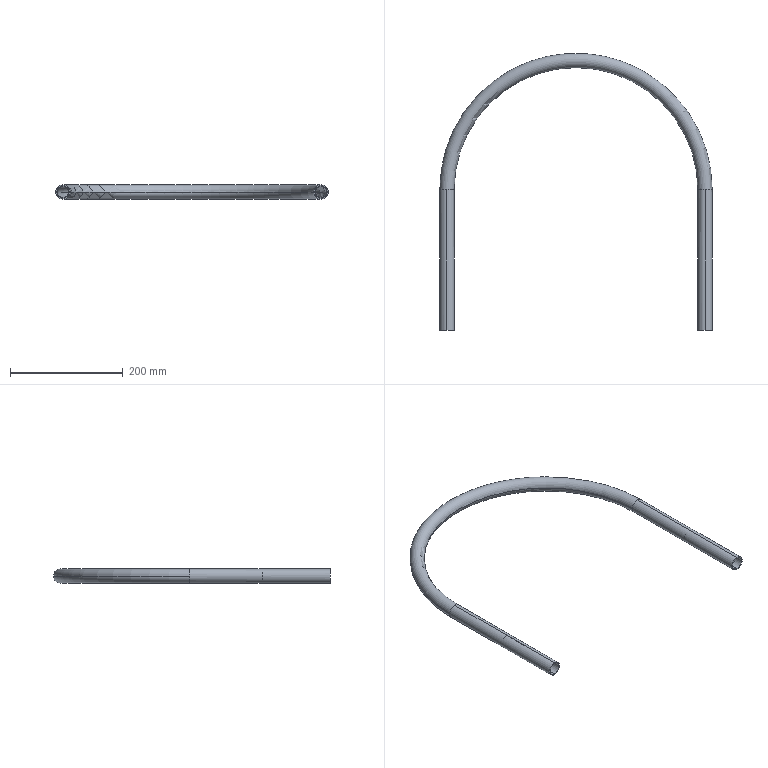Part | STEP file | 51E-01212JG10 | 1 solid | 20 faces | box 483.4 x 491.7 x 25.4 mm | volume 222157 mm3 | cylinder 12 | torus 4 | plane 4 | commonest cylinder face diameters 19.8 x4 25.4 x4 22.2 x2 22.5 x2
STEP:
#1=CARTESIAN_POINT('',(-238.9,250.,0.));
#2=VERTEX_POINT('',#1);
#3=CARTESIAN_POINT('',(-229.,250.,9.9));
#4=VERTEX_POINT('',#3);
#5=CARTESIAN_POINT('',(-229.,250.,0.));
#6=DIRECTION('',(0.,-1.,0.));
#7=AXIS2_PLACEMENT_3D('',#5,#6,$);
#8=CIRCLE('',#7,9.9);
#9=EDGE_CURVE('',#2,#4,#8,.F.);
#10=ORIENTED_EDGE('',*,*,#9,.F.);
#11=CARTESIAN_POINT('',(238.9,250.,0.));
#12=VERTEX_POINT('',#11);
#13=CARTESIAN_POINT('',(0.,250.,0.));
#14=DIRECTION('',(0.,0.,-1.));
#15=AXIS2_PLACEMENT_3D('',#13,#14,$);
#16=CIRCLE('',#15,238.9);
#17=EDGE_CURVE('',#2,#12,#16,.T.);
#18=ORIENTED_EDGE('',*,*,#17,.T.);
#19=CARTESIAN_POINT('',(229.,250.,9.9));
#20=VERTEX_POINT('',#19);
#21=CARTESIAN_POINT('',(229.,250.,0.));
#22=DIRECTION('',(0.,1.,0.));
#23=AXIS2_PLACEMENT_3D('',#21,#22,$);
#24=CIRCLE('',#23,9.9);
#25=EDGE_CURVE('',#12,#20,#24,.F.);
#26=ORIENTED_EDGE('',*,*,#25,.T.);
#27=CARTESIAN_POINT('',(219.1,250.,0.));
#28=VERTEX_POINT('',#27);
#29=CARTESIAN_POINT('',(229.,250.,0.));
#30=DIRECTION('',(0.,1.,0.));
#31=AXIS2_PLACEMENT_3D('',#29,#30,$);
#32=CIRCLE('',#31,9.9);
#33=EDGE_CURVE('',#20,#28,#32,.F.);
#34=ORIENTED_EDGE('',*,*,#33,.T.);
#35=CARTESIAN_POINT('',(-219.1,250.,0.));
#36=VERTEX_POINT('',#35);
#37=CARTESIAN_POINT('',(0.,250.,0.));
#38=DIRECTION('',(0.,0.,-1.));
#39=AXIS2_PLACEMENT_3D('',#37,#38,$);
#40=CIRCLE('',#39,219.1);
#41=EDGE_CURVE('',#36,#28,#40,.T.);
#42=ORIENTED_EDGE('',*,*,#41,.F.);
#43=CARTESIAN_POINT('',(-229.,250.,0.));
#44=DIRECTION('',(0.,-1.,0.));
#45=AXIS2_PLACEMENT_3D('',#43,#44,$);
#46=CIRCLE('',#45,9.9);
#47=EDGE_CURVE('',#4,#36,#46,.F.);
#48=ORIENTED_EDGE('',*,*,#47,.F.);
#49=EDGE_LOOP('',(#10,#18,#26,#34,#42,#48));
#50=FACE_OUTER_BOUND('',#49,.T.);
#51=CARTESIAN_POINT('',(0.,250.,0.));
#52=DIRECTION('',(0.,0.,-1.));
#53=DIRECTION('',(-1.,0.,0.));
#54=AXIS2_PLACEMENT_3D('',#51,#52,#53);
#55=TOROIDAL_SURFACE('',#54,229.,9.9);
#56=ADVANCED_FACE('',(#50),#55,.F.);
#57=CARTESIAN_POINT('',(-229.,250.,-9.9));
#58=VERTEX_POINT('',#57);
#59=CARTESIAN_POINT('',(-229.,250.,0.));
#60=DIRECTION('',(0.,-1.,0.));
#61=AXIS2_PLACEMENT_3D('',#59,#60,$);
#62=CIRCLE('',#61,9.9);
#63=EDGE_CURVE('',#58,#2,#62,.F.);
#64=ORIENTED_EDGE('',*,*,#63,.T.);
#65=ORIENTED_EDGE('',*,*,#9,.T.);
#66=CARTESIAN_POINT('',(-229.,120.,9.9));
#67=VERTEX_POINT('',#66);
#68=CARTESIAN_POINT('',(-229.,250.,9.9));
#69=DIRECTION('',(0.,-1.,0.));
#70=VECTOR('',#69,1.);
#71=LINE('',#68,#70);
#72=EDGE_CURVE('',#4,#67,#71,.T.);
#73=ORIENTED_EDGE('',*,*,#72,.T.);
#74=CARTESIAN_POINT('',(-229.,120.,-9.9));
#75=VERTEX_POINT('',#74);
#76=CARTESIAN_POINT('',(-229.,120.,0.));
#77=DIRECTION('',(0.,-1.,0.));
#78=AXIS2_PLACEMENT_3D('',#76,#77,$);
#79=CIRCLE('',#78,9.9);
#80=EDGE_CURVE('',#75,#67,#79,.F.);
#81=ORIENTED_EDGE('',*,*,#80,.F.);
#82=CARTESIAN_POINT('',(-229.,250.,-9.9));
#83=DIRECTION('',(0.,-1.,0.));
#84=VECTOR('',#83,1.);
#85=LINE('',#82,#84);
#86=EDGE_CURVE('',#58,#75,#85,.T.);
#87=ORIENTED_EDGE('',*,*,#86,.F.);
#88=EDGE_LOOP('',(#64,#65,#73,#81,#87));
#89=FACE_OUTER_BOUND('',#88,.T.);
#90=CARTESIAN_POINT('',(-229.,250.,0.));
#91=DIRECTION('',(0.,-1.,0.));
#92=DIRECTION('',(0.,0.,1.));
#93=AXIS2_PLACEMENT_3D('',#90,#91,#92);
#94=CYLINDRICAL_SURFACE('',#93,9.9);
#95=ADVANCED_FACE('',(#89),#94,.F.);
#96=ORIENTED_EDGE('',*,*,#17,.F.);
#97=ORIENTED_EDGE('',*,*,#63,.F.);
#98=CARTESIAN_POINT('',(-229.,250.,0.));
#99=DIRECTION('',(0.,-1.,0.));
#100=AXIS2_PLACEMENT_3D('',#98,#99,$);
#101=CIRCLE('',#100,9.9);
#102=EDGE_CURVE('',#36,#58,#101,.F.);
#103=ORIENTED_EDGE('',*,*,#102,.F.);
#104=ORIENTED_EDGE('',*,*,#41,.T.);
#105=CARTESIAN_POINT('',(229.,250.,-9.9));
#106=VERTEX_POINT('',#105);
#107=CARTESIAN_POINT('',(229.,250.,0.));
#108=DIRECTION('',(0.,1.,0.));
#109=AXIS2_PLACEMENT_3D('',#107,#108,$);
#110=CIRCLE('',#109,9.9);
#111=EDGE_CURVE('',#28,#106,#110,.F.);
#112=ORIENTED_EDGE('',*,*,#111,.T.);
#113=CARTESIAN_POINT('',(229.,250.,0.));
#114=DIRECTION('',(0.,1.,0.));
#115=AXIS2_PLACEMENT_3D('',#113,#114,$);
#116=CIRCLE('',#115,9.9);
#117=EDGE_CURVE('',#106,#12,#116,.F.);
#118=ORIENTED_EDGE('',*,*,#117,.T.);
#119=EDGE_LOOP('',(#96,#97,#103,#104,#112,#118));
#120=FACE_OUTER_BOUND('',#119,.T.);
#121=CARTESIAN_POINT('',(0.,250.,0.));
#122=DIRECTION('',(0.,0.,-1.));
#123=DIRECTION('',(-1.,0.,0.));
#124=AXIS2_PLACEMENT_3D('',#121,#122,#123);
#125=TOROIDAL_SURFACE('',#124,229.,9.9);
#126=ADVANCED_FACE('',(#120),#125,.F.);
#127=CARTESIAN_POINT('',(229.,120.,9.9));
#128=VERTEX_POINT('',#127);
#129=CARTESIAN_POINT('',(229.,250.,9.9));
#130=DIRECTION('',(0.,-1.,0.));
#131=VECTOR('',#130,1.);
#132=LINE('',#129,#131);
#133=EDGE_CURVE('',#20,#128,#132,.T.);
#134=ORIENTED_EDGE('',*,*,#133,.F.);
#135=ORIENTED_EDGE('',*,*,#25,.F.);
#136=ORIENTED_EDGE('',*,*,#117,.F.);
#137=CARTESIAN_POINT('',(229.,120.,-9.9));
#138=VERTEX_POINT('',#137);
#139=CARTESIAN_POINT('',(229.,250.,-9.9));
#140=DIRECTION('',(0.,-1.,0.));
#141=VECTOR('',#140,1.);
#142=LINE('',#139,#141);
#143=EDGE_CURVE('',#106,#138,#142,.T.);
#144=ORIENTED_EDGE('',*,*,#143,.T.);
#145=CARTESIAN_POINT('',(229.,120.,0.));
#146=DIRECTION('',(0.,-1.,0.));
#147=AXIS2_PLACEMENT_3D('',#145,#146,$);
#148=CIRCLE('',#147,9.9);
#149=EDGE_CURVE('',#138,#128,#148,.T.);
#150=ORIENTED_EDGE('',*,*,#149,.T.);
#151=EDGE_LOOP('',(#134,#135,#136,#144,#150));
#152=FACE_OUTER_BOUND('',#151,.T.);
#153=CARTESIAN_POINT('',(229.,250.,0.));
#154=DIRECTION('',(0.,-1.,0.));
#155=DIRECTION('',(0.,0.,-1.));
#156=AXIS2_PLACEMENT_3D('',#153,#154,#155);
#157=CYLINDRICAL_SURFACE('',#156,9.9);
#158=ADVANCED_FACE('',(#152),#157,.F.);
#159=ORIENTED_EDGE('',*,*,#33,.F.);
#160=ORIENTED_EDGE('',*,*,#133,.T.);
#161=CARTESIAN_POINT('',(229.,120.,0.));
#162=DIRECTION('',(0.,-1.,0.));
#163=AXIS2_PLACEMENT_3D('',#161,#162,$);
#164=CIRCLE('',#163,9.9);
#165=EDGE_CURVE('',#128,#138,#164,.T.);
#166=ORIENTED_EDGE('',*,*,#165,.T.);
#167=ORIENTED_EDGE('',*,*,#143,.F.);
#168=ORIENTED_EDGE('',*,*,#111,.F.);
#169=EDGE_LOOP('',(#159,#160,#166,#167,#168));
#170=FACE_OUTER_BOUND('',#169,.T.);
#171=CARTESIAN_POINT('',(229.,250.,0.));
#172=DIRECTION('',(0.,-1.,0.));
#173=DIRECTION('',(0.,0.,1.));
#174=AXIS2_PLACEMENT_3D('',#171,#172,#173);
#175=CYLINDRICAL_SURFACE('',#174,9.9);
#176=ADVANCED_FACE('',(#170),#175,.F.);
#177=ORIENTED_EDGE('',*,*,#72,.F.);
#178=ORIENTED_EDGE('',*,*,#47,.T.);
#179=ORIENTED_EDGE('',*,*,#102,.T.);
#180=ORIENTED_EDGE('',*,*,#86,.T.);
#181=CARTESIAN_POINT('',(-229.,120.,0.));
#182=DIRECTION('',(0.,-1.,0.));
#183=AXIS2_PLACEMENT_3D('',#181,#182,$);
#184=CIRCLE('',#183,9.9);
#185=EDGE_CURVE('',#67,#75,#184,.F.);
#186=ORIENTED_EDGE('',*,*,#185,.F.);
#187=EDGE_LOOP('',(#177,#178,#179,#180,#186));
#188=FACE_OUTER_BOUND('',#187,.T.);
#189=CARTESIAN_POINT('',(-229.,250.,0.));
#190=DIRECTION('',(0.,-1.,0.));
#191=DIRECTION('',(0.,0.,-1.));
#192=AXIS2_PLACEMENT_3D('',#189,#190,#191);
#193=CYLINDRICAL_SURFACE('',#192,9.9);
#194=ADVANCED_FACE('',(#188),#193,.F.);
#195=CARTESIAN_POINT('',(-229.,120.,-11.1));
#196=VERTEX_POINT('',#195);
#197=CARTESIAN_POINT('',(-229.,120.,11.1));
#198=VERTEX_POINT('',#197);
#199=CARTESIAN_POINT('',(-229.,120.,0.));
#200=DIRECTION('',(0.,1.,0.));
#201=AXIS2_PLACEMENT_3D('',#199,#200,$);
#202=CIRCLE('',#201,11.1);
#203=EDGE_CURVE('',#196,#198,#202,.T.);
#204=ORIENTED_EDGE('',*,*,#203,.F.);
#205=CARTESIAN_POINT('',(-229.,120.,0.));
#206=DIRECTION('',(0.,1.,0.));
#207=AXIS2_PLACEMENT_3D('',#205,#206,$);
#208=CIRCLE('',#207,11.1);
#209=EDGE_CURVE('',#198,#196,#208,.T.);
#210=ORIENTED_EDGE('',*,*,#209,.F.);
#211=EDGE_LOOP('',(#204,#210));
#212=FACE_OUTER_BOUND('',#211,.T.);
#213=ORIENTED_EDGE('',*,*,#80,.T.);
#214=ORIENTED_EDGE('',*,*,#185,.T.);
#215=EDGE_LOOP('',(#213,#214));
#216=FACE_BOUND('',#215,.T.);
#217=CARTESIAN_POINT('',(-229.,120.,0.));
#218=DIRECTION('',(0.,1.,0.));
#219=DIRECTION('',(0.,0.,1.));
#220=AXIS2_PLACEMENT_3D('',#217,#218,#219);
#221=PLANE('',#220);
#222=ADVANCED_FACE('',(#212,#216),#221,.F.);
#223=CARTESIAN_POINT('',(229.,120.,-11.25));
#224=VERTEX_POINT('',#223);
#225=CARTESIAN_POINT('',(229.,120.,11.25));
#226=VERTEX_POINT('',#225);
#227=CARTESIAN_POINT('',(229.,120.,0.));
#228=DIRECTION('',(0.,1.,0.));
#229=AXIS2_PLACEMENT_3D('',#227,#228,$);
#230=CIRCLE('',#229,11.25);
#231=EDGE_CURVE('',#224,#226,#230,.T.);
#232=ORIENTED_EDGE('',*,*,#231,.F.);
#233=CARTESIAN_POINT('',(229.,120.,0.));
#234=DIRECTION('',(0.,1.,0.));
#235=AXIS2_PLACEMENT_3D('',#233,#234,$);
#236=CIRCLE('',#235,11.25);
#237=EDGE_CURVE('',#226,#224,#236,.T.);
#238=ORIENTED_EDGE('',*,*,#237,.F.);
#239=EDGE_LOOP('',(#232,#238));
#240=FACE_OUTER_BOUND('',#239,.T.);
#241=ORIENTED_EDGE('',*,*,#149,.F.);
#242=ORIENTED_EDGE('',*,*,#165,.F.);
#243=EDGE_LOOP('',(#241,#242));
#244=FACE_BOUND('',#243,.T.);
#245=CARTESIAN_POINT('',(229.,120.,0.));
#246=DIRECTION('',(0.,1.,0.));
#247=DIRECTION('',(0.,0.,1.));
#248=AXIS2_PLACEMENT_3D('',#245,#246,#247);
#249=PLANE('',#248);
#250=ADVANCED_FACE('',(#240,#244),#249,.F.);
#251=ORIENTED_EDGE('',*,*,#203,.T.);
#252=CARTESIAN_POINT('',(-229.,0.,11.1));
#253=VERTEX_POINT('',#252);
#254=CARTESIAN_POINT('',(-229.,120.,11.1));
#255=DIRECTION('',(0.,-1.,0.));
#256=VECTOR('',#255,1.);
#257=LINE('',#254,#256);
#258=EDGE_CURVE('',#198,#253,#257,.T.);
#259=ORIENTED_EDGE('',*,*,#258,.T.);
#260=CARTESIAN_POINT('',(-229.,0.,-11.1));
#261=VERTEX_POINT('',#260);
#262=CARTESIAN_POINT('',(-229.,0.,0.));
#263=DIRECTION('',(0.,-1.,0.));
#264=AXIS2_PLACEMENT_3D('',#262,#263,$);
#265=CIRCLE('',#264,11.1);
#266=EDGE_CURVE('',#261,#253,#265,.F.);
#267=ORIENTED_EDGE('',*,*,#266,.F.);
#268=CARTESIAN_POINT('',(-229.,120.,-11.1));
#269=DIRECTION('',(0.,-1.,0.));
#270=VECTOR('',#269,1.);
#271=LINE('',#268,#270);
#272=EDGE_CURVE('',#196,#261,#271,.T.);
#273=ORIENTED_EDGE('',*,*,#272,.F.);
#274=EDGE_LOOP('',(#251,#259,#267,#273));
#275=FACE_OUTER_BOUND('',#274,.T.);
#276=CARTESIAN_POINT('',(-229.,120.,0.));
#277=DIRECTION('',(0.,-1.,0.));
#278=DIRECTION('',(0.,0.,1.));
#279=AXIS2_PLACEMENT_3D('',#276,#277,#278);
#280=CYLINDRICAL_SURFACE('',#279,11.1);
#281=ADVANCED_FACE('',(#275),#280,.F.);
#282=ORIENTED_EDGE('',*,*,#258,.F.);
#283=ORIENTED_EDGE('',*,*,#209,.T.);
#284=ORIENTED_EDGE('',*,*,#272,.T.);
#285=CARTESIAN_POINT('',(-229.,0.,0.));
#286=DIRECTION('',(0.,-1.,0.));
#287=AXIS2_PLACEMENT_3D('',#285,#286,$);
#288=CIRCLE('',#287,11.1);
#289=EDGE_CURVE('',#253,#261,#288,.F.);
#290=ORIENTED_EDGE('',*,*,#289,.F.);
#291=EDGE_LOOP('',(#282,#283,#284,#290));
#292=FACE_OUTER_BOUND('',#291,.T.);
#293=CARTESIAN_POINT('',(-229.,120.,0.));
#294=DIRECTION('',(0.,-1.,0.));
#295=DIRECTION('',(0.,0.,-1.));
#296=AXIS2_PLACEMENT_3D('',#293,#294,#295);
#297=CYLINDRICAL_SURFACE('',#296,11.1);
#298=ADVANCED_FACE('',(#292),#297,.F.);
#299=ORIENTED_EDGE('',*,*,#231,.T.);
#300=CARTESIAN_POINT('',(229.,0.,11.25));
#301=VERTEX_POINT('',#300);
#302=CARTESIAN_POINT('',(229.,120.,11.25));
#303=DIRECTION('',(0.,-1.,0.));
#304=VECTOR('',#303,1.);
#305=LINE('',#302,#304);
#306=EDGE_CURVE('',#226,#301,#305,.T.);
#307=ORIENTED_EDGE('',*,*,#306,.T.);
#308=CARTESIAN_POINT('',(229.,0.,-11.25));
#309=VERTEX_POINT('',#308);
#310=CARTESIAN_POINT('',(229.,0.,0.));
#311=DIRECTION('',(0.,-1.,0.));
#312=AXIS2_PLACEMENT_3D('',#310,#311,$);
#313=CIRCLE('',#312,11.25);
#314=EDGE_CURVE('',#309,#301,#313,.F.);
#315=ORIENTED_EDGE('',*,*,#314,.F.);
#316=CARTESIAN_POINT('',(229.,120.,-11.25));
#317=DIRECTION('',(0.,-1.,0.));
#318=VECTOR('',#317,1.);
#319=LINE('',#316,#318);
#320=EDGE_CURVE('',#224,#309,#319,.T.);
#321=ORIENTED_EDGE('',*,*,#320,.F.);
#322=EDGE_LOOP('',(#299,#307,#315,#321));
#323=FACE_OUTER_BOUND('',#322,.T.);
#324=CARTESIAN_POINT('',(229.,120.,0.));
#325=DIRECTION('',(0.,-1.,0.));
#326=DIRECTION('',(0.,0.,1.));
#327=AXIS2_PLACEMENT_3D('',#324,#325,#326);
#328=CYLINDRICAL_SURFACE('',#327,11.25);
#329=ADVANCED_FACE('',(#323),#328,.F.);
#330=ORIENTED_EDGE('',*,*,#306,.F.);
#331=ORIENTED_EDGE('',*,*,#237,.T.);
#332=ORIENTED_EDGE('',*,*,#320,.T.);
#333=CARTESIAN_POINT('',(229.,0.,0.));
#334=DIRECTION('',(0.,-1.,0.));
#335=AXIS2_PLACEMENT_3D('',#333,#334,$);
#336=CIRCLE('',#335,11.25);
#337=EDGE_CURVE('',#301,#309,#336,.F.);
#338=ORIENTED_EDGE('',*,*,#337,.F.);
#339=EDGE_LOOP('',(#330,#331,#332,#338));
#340=FACE_OUTER_BOUND('',#339,.T.);
#341=CARTESIAN_POINT('',(229.,120.,0.));
#342=DIRECTION('',(0.,-1.,0.));
#343=DIRECTION('',(0.,0.,-1.));
#344=AXIS2_PLACEMENT_3D('',#341,#342,#343);
#345=CYLINDRICAL_SURFACE('',#344,11.25);
#346=ADVANCED_FACE('',(#340),#345,.F.);
#347=CARTESIAN_POINT('',(-229.,0.,-12.7));
#348=VERTEX_POINT('',#347);
#349=CARTESIAN_POINT('',(-229.,0.,12.7));
#350=VERTEX_POINT('',#349);
#351=CARTESIAN_POINT('',(-229.,0.,0.));
#352=DIRECTION('',(0.,1.,0.));
#353=AXIS2_PLACEMENT_3D('',#351,#352,$);
#354=CIRCLE('',#353,12.7);
#355=EDGE_CURVE('',#348,#350,#354,.T.);
#356=ORIENTED_EDGE('',*,*,#355,.F.);
#357=CARTESIAN_POINT('',(-229.,0.,0.));
#358=DIRECTION('',(0.,1.,0.));
#359=AXIS2_PLACEMENT_3D('',#357,#358,$);
#360=CIRCLE('',#359,12.7);
#361=EDGE_CURVE('',#350,#348,#360,.T.);
#362=ORIENTED_EDGE('',*,*,#361,.F.);
#363=EDGE_LOOP('',(#356,#362));
#364=FACE_OUTER_BOUND('',#363,.T.);
#365=ORIENTED_EDGE('',*,*,#266,.T.);
#366=ORIENTED_EDGE('',*,*,#289,.T.);
#367=EDGE_LOOP('',(#365,#366));
#368=FACE_BOUND('',#367,.T.);
#369=CARTESIAN_POINT('',(-229.,0.,0.));
#370=DIRECTION('',(0.,1.,0.));
#371=DIRECTION('',(0.,0.,1.));
#372=AXIS2_PLACEMENT_3D('',#369,#370,#371);
#373=PLANE('',#372);
#374=ADVANCED_FACE('',(#364,#368),#373,.F.);
#375=CARTESIAN_POINT('',(229.,0.,-12.7));
#376=VERTEX_POINT('',#375);
#377=CARTESIAN_POINT('',(229.,0.,12.7));
#378=VERTEX_POINT('',#377);
#379=CARTESIAN_POINT('',(229.,0.,0.));
#380=DIRECTION('',(0.,-1.,0.));
#381=AXIS2_PLACEMENT_3D('',#379,#380,$);
#382=CIRCLE('',#381,12.7);
#383=EDGE_CURVE('',#376,#378,#382,.T.);
#384=ORIENTED_EDGE('',*,*,#383,.T.);
#385=CARTESIAN_POINT('',(229.,0.,0.));
#386=DIRECTION('',(0.,-1.,0.));
#387=AXIS2_PLACEMENT_3D('',#385,#386,$);
#388=CIRCLE('',#387,12.7);
#389=EDGE_CURVE('',#378,#376,#388,.T.);
#390=ORIENTED_EDGE('',*,*,#389,.T.);
#391=EDGE_LOOP('',(#384,#390));
#392=FACE_OUTER_BOUND('',#391,.T.);
#393=ORIENTED_EDGE('',*,*,#314,.T.);
#394=ORIENTED_EDGE('',*,*,#337,.T.);
#395=EDGE_LOOP('',(#393,#394));
#396=FACE_BOUND('',#395,.T.);
#397=CARTESIAN_POINT('',(229.,0.,0.));
#398=DIRECTION('',(0.,-1.,0.));
#399=DIRECTION('',(0.,0.,1.));
#400=AXIS2_PLACEMENT_3D('',#397,#398,#399);
#401=PLANE('',#400);
#402=ADVANCED_FACE('',(#392,#396),#401,.T.);
#403=CARTESIAN_POINT('',(-229.,250.,12.7));
#404=VERTEX_POINT('',#403);
#405=CARTESIAN_POINT('',(-229.,250.,12.7));
#406=DIRECTION('',(0.,-1.,0.));
#407=VECTOR('',#406,1.);
#408=LINE('',#405,#407);
#409=EDGE_CURVE('',#404,#350,#408,.T.);
#410=ORIENTED_EDGE('',*,*,#409,.F.);
#411=CARTESIAN_POINT('',(-241.7,250.,0.));
#412=VERTEX_POINT('',#411);
#413=CARTESIAN_POINT('',(-229.,250.,0.));
#414=DIRECTION('',(0.,-1.,0.));
#415=AXIS2_PLACEMENT_3D('',#413,#414,$);
#416=CIRCLE('',#415,12.7);
#417=EDGE_CURVE('',#412,#404,#416,.F.);
#418=ORIENTED_EDGE('',*,*,#417,.F.);
#419=CARTESIAN_POINT('',(-229.,250.,-12.7));
#420=VERTEX_POINT('',#419);
#421=CARTESIAN_POINT('',(-229.,250.,0.));
#422=DIRECTION('',(0.,-1.,0.));
#423=AXIS2_PLACEMENT_3D('',#421,#422,$);
#424=CIRCLE('',#423,12.7);
#425=EDGE_CURVE('',#420,#412,#424,.F.);
#426=ORIENTED_EDGE('',*,*,#425,.F.);
#427=CARTESIAN_POINT('',(-229.,250.,-12.7));
#428=DIRECTION('',(0.,-1.,0.));
#429=VECTOR('',#428,1.);
#430=LINE('',#427,#429);
#431=EDGE_CURVE('',#420,#348,#430,.T.);
#432=ORIENTED_EDGE('',*,*,#431,.T.);
#433=ORIENTED_EDGE('',*,*,#355,.T.);
#434=EDGE_LOOP('',(#410,#418,#426,#432,#433));
#435=FACE_OUTER_BOUND('',#434,.T.);
#436=CARTESIAN_POINT('',(-229.,250.,0.));
#437=DIRECTION('',(0.,-1.,0.));
#438=DIRECTION('',(0.,0.,1.));
#439=AXIS2_PLACEMENT_3D('',#436,#437,#438);
#440=CYLINDRICAL_SURFACE('',#439,12.7);
#441=ADVANCED_FACE('',(#435),#440,.T.);
#442=CARTESIAN_POINT('',(-216.3,250.,0.));
#443=VERTEX_POINT('',#442);
#444=CARTESIAN_POINT('',(-229.,250.,0.));
#445=DIRECTION('',(0.,-1.,0.));
#446=AXIS2_PLACEMENT_3D('',#444,#445,$);
#447=CIRCLE('',#446,12.7);
#448=EDGE_CURVE('',#404,#443,#447,.F.);
#449=ORIENTED_EDGE('',*,*,#448,.F.);
#450=ORIENTED_EDGE('',*,*,#409,.T.);
#451=ORIENTED_EDGE('',*,*,#361,.T.);
#452=ORIENTED_EDGE('',*,*,#431,.F.);
#453=CARTESIAN_POINT('',(-229.,250.,0.));
#454=DIRECTION('',(0.,-1.,0.));
#455=AXIS2_PLACEMENT_3D('',#453,#454,$);
#456=CIRCLE('',#455,12.7);
#457=EDGE_CURVE('',#443,#420,#456,.F.);
#458=ORIENTED_EDGE('',*,*,#457,.F.);
#459=EDGE_LOOP('',(#449,#450,#451,#452,#458));
#460=FACE_OUTER_BOUND('',#459,.T.);
#461=CARTESIAN_POINT('',(-229.,250.,0.));
#462=DIRECTION('',(0.,-1.,0.));
#463=DIRECTION('',(0.,0.,-1.));
#464=AXIS2_PLACEMENT_3D('',#461,#462,#463);
#465=CYLINDRICAL_SURFACE('',#464,12.7);
#466=ADVANCED_FACE('',(#460),#465,.T.);
#467=CARTESIAN_POINT('',(229.,250.,-12.7));
#468=VERTEX_POINT('',#467);
#469=CARTESIAN_POINT('',(241.7,250.,0.));
#470=VERTEX_POINT('',#469);
#471=CARTESIAN_POINT('',(229.,250.,0.));
#472=DIRECTION('',(0.,-1.,0.));
#473=AXIS2_PLACEMENT_3D('',#471,#472,$);
#474=CIRCLE('',#473,12.7);
#475=EDGE_CURVE('',#468,#470,#474,.T.);
#476=ORIENTED_EDGE('',*,*,#475,.T.);
#477=CARTESIAN_POINT('',(229.,250.,12.7));
#478=VERTEX_POINT('',#477);
#479=CARTESIAN_POINT('',(229.,250.,0.));
#480=DIRECTION('',(0.,-1.,0.));
#481=AXIS2_PLACEMENT_3D('',#479,#480,$);
#482=CIRCLE('',#481,12.7);
#483=EDGE_CURVE('',#470,#478,#482,.T.);
#484=ORIENTED_EDGE('',*,*,#483,.T.);
#485=CARTESIAN_POINT('',(229.,250.,12.7));
#486=DIRECTION('',(0.,-1.,0.));
#487=VECTOR('',#486,1.);
#488=LINE('',#485,#487);
#489=EDGE_CURVE('',#478,#378,#488,.T.);
#490=ORIENTED_EDGE('',*,*,#489,.T.);
#491=ORIENTED_EDGE('',*,*,#383,.F.);
#492=CARTESIAN_POINT('',(229.,250.,-12.7));
#493=DIRECTION('',(0.,-1.,0.));
#494=VECTOR('',#493,1.);
#495=LINE('',#492,#494);
#496=EDGE_CURVE('',#468,#376,#495,.T.);
#497=ORIENTED_EDGE('',*,*,#496,.F.);
#498=EDGE_LOOP('',(#476,#484,#490,#491,#497));
#499=FACE_OUTER_BOUND('',#498,.T.);
#500=CARTESIAN_POINT('',(229.,250.,0.));
#501=DIRECTION('',(0.,-1.,0.));
#502=DIRECTION('',(0.,0.,-1.));
#503=AXIS2_PLACEMENT_3D('',#500,#501,#502);
#504=CYLINDRICAL_SURFACE('',#503,12.7);
#505=ADVANCED_FACE('',(#499),#504,.T.);
#506=ORIENTED_EDGE('',*,*,#489,.F.);
#507=CARTESIAN_POINT('',(216.3,250.,0.));
#508=VERTEX_POINT('',#507);
#509=CARTESIAN_POINT('',(229.,250.,0.));
#510=DIRECTION('',(0.,-1.,0.));
#511=AXIS2_PLACEMENT_3D('',#509,#510,$);
#512=CIRCLE('',#511,12.7);
#513=EDGE_CURVE('',#478,#508,#512,.T.);
#514=ORIENTED_EDGE('',*,*,#513,.T.);
#515=CARTESIAN_POINT('',(229.,250.,0.));
#516=DIRECTION('',(0.,-1.,0.));
#517=AXIS2_PLACEMENT_3D('',#515,#516,$);
#518=CIRCLE('',#517,12.7);
#519=EDGE_CURVE('',#508,#468,#518,.T.);
#520=ORIENTED_EDGE('',*,*,#519,.T.);
#521=ORIENTED_EDGE('',*,*,#496,.T.);
#522=ORIENTED_EDGE('',*,*,#389,.F.);
#523=EDGE_LOOP('',(#506,#514,#520,#521,#522));
#524=FACE_OUTER_BOUND('',#523,.T.);
#525=CARTESIAN_POINT('',(229.,250.,0.));
#526=DIRECTION('',(0.,-1.,0.));
#527=DIRECTION('',(0.,0.,1.));
#528=AXIS2_PLACEMENT_3D('',#525,#526,#527);
#529=CYLINDRICAL_SURFACE('',#528,12.7);
#530=ADVANCED_FACE('',(#524),#529,.T.);
#531=CARTESIAN_POINT('',(0.,250.,0.));
#532=DIRECTION('',(0.,0.,-1.));
#533=AXIS2_PLACEMENT_3D('',#531,#532,$);
#534=CIRCLE('',#533,241.7);
#535=EDGE_CURVE('',#412,#470,#534,.T.);
#536=ORIENTED_EDGE('',*,*,#535,.F.);
#537=ORIENTED_EDGE('',*,*,#417,.T.);
#538=ORIENTED_EDGE('',*,*,#448,.T.);
#539=CARTESIAN_POINT('',(0.,250.,0.));
#540=DIRECTION('',(0.,0.,-1.));
#541=AXIS2_PLACEMENT_3D('',#539,#540,$);
#542=CIRCLE('',#541,216.3);
#543=EDGE_CURVE('',#443,#508,#542,.T.);
#544=ORIENTED_EDGE('',*,*,#543,.T.);
#545=ORIENTED_EDGE('',*,*,#513,.F.);
#546=ORIENTED_EDGE('',*,*,#483,.F.);
#547=EDGE_LOOP('',(#536,#537,#538,#544,#545,#546));
#548=FACE_OUTER_BOUND('',#547,.T.);
#549=CARTESIAN_POINT('',(0.,250.,0.));
#550=DIRECTION('',(0.,0.,-1.));
#551=DIRECTION('',(-1.,0.,0.));
#552=AXIS2_PLACEMENT_3D('',#549,#550,#551);
#553=TOROIDAL_SURFACE('',#552,229.,12.7);
#554=ADVANCED_FACE('',(#548),#553,.T.);
#555=ORIENTED_EDGE('',*,*,#425,.T.);
#556=ORIENTED_EDGE('',*,*,#535,.T.);
#557=ORIENTED_EDGE('',*,*,#475,.F.);
#558=ORIENTED_EDGE('',*,*,#519,.F.);
#559=ORIENTED_EDGE('',*,*,#543,.F.);
#560=ORIENTED_EDGE('',*,*,#457,.T.);
#561=EDGE_LOOP('',(#555,#556,#557,#558,#559,#560));
#562=FACE_OUTER_BOUND('',#561,.T.);
#563=CARTESIAN_POINT('',(0.,250.,0.));
#564=DIRECTION('',(0.,0.,-1.));
#565=DIRECTION('',(-1.,0.,0.));
#566=AXIS2_PLACEMENT_3D('',#563,#564,#565);
#567=TOROIDAL_SURFACE('',#566,229.,12.7);
#568=ADVANCED_FACE('',(#562),#567,.T.);
#569=CLOSED_SHELL('',(#56,#95,#126,#158,#176,#194,#222,#250,#281,#298,#329,#346,#374,#402,#441,#466,#505,#530,#554,#568));
#570=MANIFOLD_SOLID_BREP('',#569);
#571=(LENGTH_UNIT()NAMED_UNIT(*)SI_UNIT(.MILLI.,.METRE.));
#572=UNCERTAINTY_MEASURE_WITH_UNIT(LENGTH_MEASURE(0.005),#571,'','');
#573=(NAMED_UNIT(*)PLANE_ANGLE_UNIT()SI_UNIT($,.RADIAN.));
#574=(NAMED_UNIT(*)SI_UNIT($,.STERADIAN.)SOLID_ANGLE_UNIT());
#575=(GEOMETRIC_REPRESENTATION_CONTEXT(3)GLOBAL_UNCERTAINTY_ASSIGNED_CONTEXT((#572))GLOBAL_UNIT_ASSIGNED_CONTEXT((#571,#573,#574))REPRESENTATION_CONTEXT('',''));
#576=ADVANCED_BREP_SHAPE_REPRESENTATION('',(#570),#575);